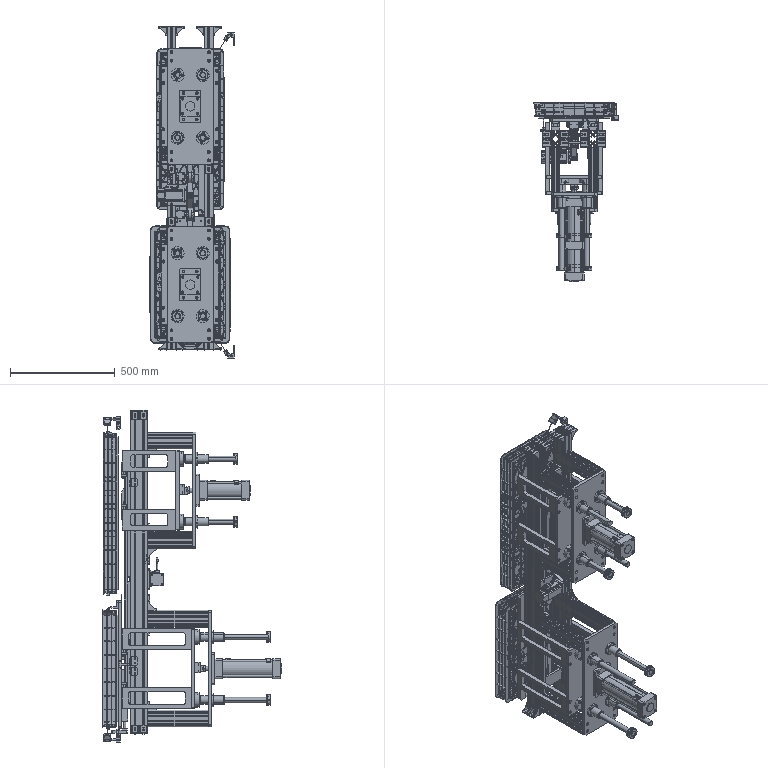Part | SolidWorks | 218 solids | 19338 faces | volume 31067630 mm3 | plane 10606 | cylinder 6069 | cone 1291 | spline 1209 | torus 147 | sphere 16 | commonest cylinder face diameters 4 x477 9 x405 2 x316 1 x252 4.2 x234 8.5 x198